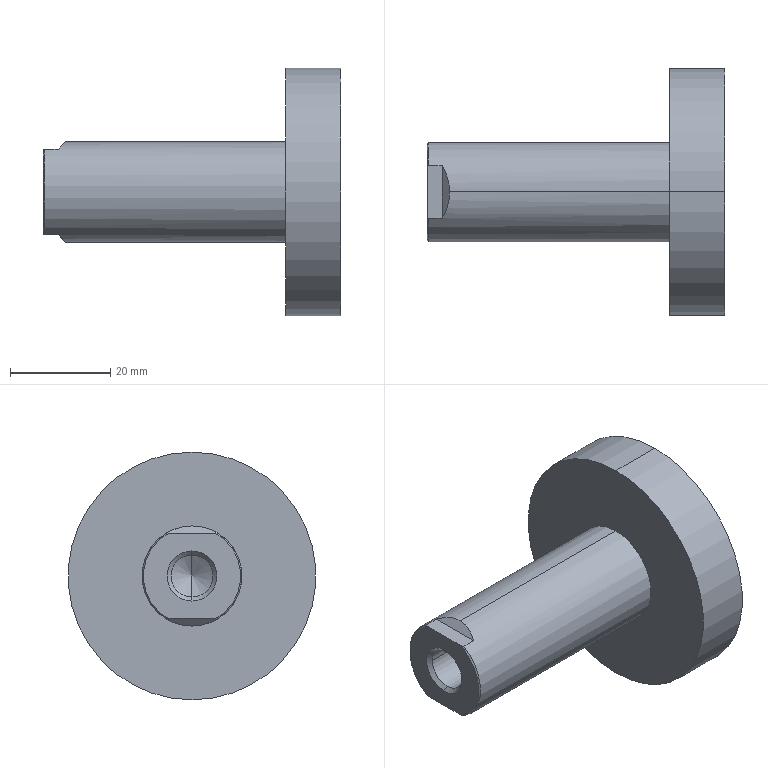Part | SolidWorks | features BaseBody 1 | 1 solid | 19 faces | box 59.5 x 49.5 x 49.5 mm | volume 35281 mm3 | plane 7 | cylinder 6 | cone 6 | commonest cylinder face diameters 8.376 x2 20 x2 49.5 x2
STEP:
#1=CARTESIAN_POINT('',(39.5,0.,10.));
#2=VERTEX_POINT('',#1);
#3=CARTESIAN_POINT('',(39.5,0.,-10.));
#4=VERTEX_POINT('',#3);
#5=CARTESIAN_POINT('',(39.5,0.,0.));
#6=DIRECTION('',(-1.,0.,0.));
#7=DIRECTION('',(0.,0.,1.));
#8=AXIS2_PLACEMENT_3D('',#5,#6,#7);
#9=CIRCLE('',#8,10.);
#10=EDGE_CURVE('',#2,#4,#9,.T.);
#11=ORIENTED_EDGE('',*,*,#10,.T.);
#12=CARTESIAN_POINT('',(-4.5,0.,-10.));
#13=VERTEX_POINT('',#12);
#14=CARTESIAN_POINT('',(0.,0.,-10.));
#15=DIRECTION('',(-1.,0.,0.));
#16=VECTOR('',#15,1000.);
#17=LINE('',#14,#16);
#18=EDGE_CURVE('',#4,#13,#17,.T.);
#19=ORIENTED_EDGE('',*,*,#18,.T.);
#20=CARTESIAN_POINT('',(-6.,5.268,-8.5));
#21=VERTEX_POINT('',#20);
#22=CARTESIAN_POINT('',(-4.5,0.,-10.));
#23=CARTESIAN_POINT('',(-4.5,1.873,-10.));
#24=CARTESIAN_POINT('',(-5.013,3.675,-9.487));
#25=CARTESIAN_POINT('',(-6.,5.268,-8.5));
#26=(BOUNDED_CURVE()B_SPLINE_CURVE(3,(#22,#23,#24,#25),.UNSPECIFIED.,.F.,.F.)B_SPLINE_CURVE_WITH_KNOTS((4,4),(3.142,3.696),.UNSPECIFIED.)CURVE()GEOMETRIC_REPRESENTATION_ITEM()RATIONAL_B_SPLINE_CURVE((1.,0.9745,0.9745,1.))REPRESENTATION_ITEM(''));
#27=EDGE_CURVE('',#13,#21,#26,.T.);
#28=ORIENTED_EDGE('',*,*,#27,.T.);
#29=CARTESIAN_POINT('',(-8.75,5.268,-8.5));
#30=VERTEX_POINT('',#29);
#31=CARTESIAN_POINT('',(0.,5.268,-8.5));
#32=DIRECTION('',(-1.,0.,0.));
#33=VECTOR('',#32,1000.);
#34=LINE('',#31,#33);
#35=EDGE_CURVE('',#21,#30,#34,.T.);
#36=ORIENTED_EDGE('',*,*,#35,.T.);
#37=CARTESIAN_POINT('',(-8.75,5.268,8.5));
#38=VERTEX_POINT('',#37);
#39=CARTESIAN_POINT('',(-8.75,0.,0.));
#40=DIRECTION('',(1.,0.,0.));
#41=DIRECTION('',(0.,0.,1.));
#42=AXIS2_PLACEMENT_3D('',#39,#40,#41);
#43=CIRCLE('',#42,10.);
#44=EDGE_CURVE('',#30,#38,#43,.T.);
#45=ORIENTED_EDGE('',*,*,#44,.T.);
#46=CARTESIAN_POINT('',(-6.,5.268,8.5));
#47=VERTEX_POINT('',#46);
#48=CARTESIAN_POINT('',(0.,5.268,8.5));
#49=DIRECTION('',(1.,0.,0.));
#50=VECTOR('',#49,1000.);
#51=LINE('',#48,#50);
#52=EDGE_CURVE('',#38,#47,#51,.T.);
#53=ORIENTED_EDGE('',*,*,#52,.T.);
#54=CARTESIAN_POINT('',(-4.5,0.,10.));
#55=VERTEX_POINT('',#54);
#56=CARTESIAN_POINT('',(-6.,5.268,8.5));
#57=CARTESIAN_POINT('',(-5.013,3.675,9.487));
#58=CARTESIAN_POINT('',(-4.5,1.873,10.));
#59=CARTESIAN_POINT('',(-4.5,0.,10.));
#60=(BOUNDED_CURVE()B_SPLINE_CURVE(3,(#56,#57,#58,#59),.UNSPECIFIED.,.F.,.F.)B_SPLINE_CURVE_WITH_KNOTS((4,4),(2.587,3.142),.UNSPECIFIED.)CURVE()GEOMETRIC_REPRESENTATION_ITEM()RATIONAL_B_SPLINE_CURVE((1.,0.9745,0.9745,1.))REPRESENTATION_ITEM(''));
#61=EDGE_CURVE('',#47,#55,#60,.T.);
#62=ORIENTED_EDGE('',*,*,#61,.T.);
#63=CARTESIAN_POINT('',(0.,0.,10.));
#64=DIRECTION('',(-1.,0.,0.));
#65=VECTOR('',#64,1000.);
#66=LINE('',#63,#65);
#67=EDGE_CURVE('',#2,#55,#66,.T.);
#68=ORIENTED_EDGE('',*,*,#67,.F.);
#69=EDGE_LOOP('',(#11,#19,#28,#36,#45,#53,#62,#68));
#70=FACE_OUTER_BOUND('',#69,.T.);
#71=CARTESIAN_POINT('',(0.,0.,0.));
#72=DIRECTION('',(-1.,0.,0.));
#73=DIRECTION('',(0.,0.,1.));
#74=AXIS2_PLACEMENT_3D('',#71,#72,#73);
#75=CYLINDRICAL_SURFACE('',#74,10.);
#76=ADVANCED_FACE('',(#70),#75,.T.);
#77=CARTESIAN_POINT('',(50.5,0.,24.75));
#78=VERTEX_POINT('',#77);
#79=CARTESIAN_POINT('',(50.5,0.,-24.75));
#80=VERTEX_POINT('',#79);
#81=CARTESIAN_POINT('',(50.5,0.,0.));
#82=DIRECTION('',(-1.,0.,0.));
#83=DIRECTION('',(0.,0.,1.));
#84=AXIS2_PLACEMENT_3D('',#81,#82,#83);
#85=CIRCLE('',#84,24.75);
#86=EDGE_CURVE('',#78,#80,#85,.T.);
#87=ORIENTED_EDGE('',*,*,#86,.T.);
#88=CARTESIAN_POINT('',(39.5,0.,-24.75));
#89=VERTEX_POINT('',#88);
#90=CARTESIAN_POINT('',(50.5,0.,-24.75));
#91=DIRECTION('',(-1.,0.,0.));
#92=VECTOR('',#91,1000.);
#93=LINE('',#90,#92);
#94=EDGE_CURVE('',#80,#89,#93,.T.);
#95=ORIENTED_EDGE('',*,*,#94,.T.);
#96=CARTESIAN_POINT('',(39.5,0.,24.75));
#97=VERTEX_POINT('',#96);
#98=CARTESIAN_POINT('',(39.5,0.,0.));
#99=DIRECTION('',(1.,0.,0.));
#100=DIRECTION('',(0.,0.,1.));
#101=AXIS2_PLACEMENT_3D('',#98,#99,#100);
#102=CIRCLE('',#101,24.75);
#103=EDGE_CURVE('',#89,#97,#102,.T.);
#104=ORIENTED_EDGE('',*,*,#103,.T.);
#105=CARTESIAN_POINT('',(50.5,0.,24.75));
#106=DIRECTION('',(-1.,0.,0.));
#107=VECTOR('',#106,1000.);
#108=LINE('',#105,#107);
#109=EDGE_CURVE('',#78,#97,#108,.T.);
#110=ORIENTED_EDGE('',*,*,#109,.F.);
#111=EDGE_LOOP('',(#87,#95,#104,#110));
#112=FACE_OUTER_BOUND('',#111,.T.);
#113=CARTESIAN_POINT('',(50.5,0.,0.));
#114=DIRECTION('',(-1.,0.,0.));
#115=DIRECTION('',(0.,0.,1.));
#116=AXIS2_PLACEMENT_3D('',#113,#114,#115);
#117=CYLINDRICAL_SURFACE('',#116,24.75);
#118=ADVANCED_FACE('',(#112),#117,.T.);
#119=CARTESIAN_POINT('',(-8.188,0.,-4.188));
#120=VERTEX_POINT('',#119);
#121=CARTESIAN_POINT('',(-8.188,-4.188,0.));
#122=VERTEX_POINT('',#121);
#123=CARTESIAN_POINT('',(-8.188,0.,0.));
#124=DIRECTION('',(-1.,0.,0.));
#125=DIRECTION('',(0.,-1.,0.));
#126=AXIS2_PLACEMENT_3D('',#123,#124,#125);
#127=CIRCLE('',#126,4.188);
#128=EDGE_CURVE('',#120,#122,#127,.T.);
#129=ORIENTED_EDGE('',*,*,#128,.F.);
#130=CARTESIAN_POINT('',(-9.,0.,-5.));
#131=VERTEX_POINT('',#130);
#132=CARTESIAN_POINT('',(-9.,0.,-5.));
#133=DIRECTION('',(-0.7071,0.,-0.7071));
#134=VECTOR('',#133,1000.);
#135=LINE('',#132,#134);
#136=EDGE_CURVE('',#120,#131,#135,.T.);
#137=ORIENTED_EDGE('',*,*,#136,.T.);
#138=CARTESIAN_POINT('',(-9.,0.,5.));
#139=VERTEX_POINT('',#138);
#140=CARTESIAN_POINT('',(-9.,0.,0.));
#141=DIRECTION('',(-1.,0.,0.));
#142=DIRECTION('',(0.,0.,1.));
#143=AXIS2_PLACEMENT_3D('',#140,#141,#142);
#144=CIRCLE('',#143,5.);
#145=EDGE_CURVE('',#131,#139,#144,.T.);
#146=ORIENTED_EDGE('',*,*,#145,.T.);
#147=CARTESIAN_POINT('',(-8.188,0.,4.188));
#148=VERTEX_POINT('',#147);
#149=CARTESIAN_POINT('',(-9.,0.,5.));
#150=DIRECTION('',(-0.7071,0.,0.7071));
#151=VECTOR('',#150,1000.);
#152=LINE('',#149,#151);
#153=EDGE_CURVE('',#148,#139,#152,.T.);
#154=ORIENTED_EDGE('',*,*,#153,.F.);
#155=CARTESIAN_POINT('',(-8.188,0.,0.));
#156=DIRECTION('',(-1.,0.,0.));
#157=DIRECTION('',(0.,-1.,0.));
#158=AXIS2_PLACEMENT_3D('',#155,#156,#157);
#159=CIRCLE('',#158,4.188);
#160=EDGE_CURVE('',#122,#148,#159,.T.);
#161=ORIENTED_EDGE('',*,*,#160,.F.);
#162=EDGE_LOOP('',(#129,#137,#146,#154,#161));
#163=FACE_OUTER_BOUND('',#162,.T.);
#164=CARTESIAN_POINT('',(-9.,0.,0.));
#165=DIRECTION('',(-1.,0.,0.));
#166=DIRECTION('',(0.,0.,1.));
#167=AXIS2_PLACEMENT_3D('',#164,#165,#166);
#168=CONICAL_SURFACE('',#167,5.,0.7854);
#169=ADVANCED_FACE('',(#163),#168,.F.);
#170=CARTESIAN_POINT('',(9.,4.188,0.));
#171=VERTEX_POINT('',#170);
#172=CARTESIAN_POINT('',(9.,0.,-4.188));
#173=VERTEX_POINT('',#172);
#174=CARTESIAN_POINT('',(9.,0.,0.));
#175=DIRECTION('',(-1.,0.,0.));
#176=DIRECTION('',(0.,-1.,0.));
#177=AXIS2_PLACEMENT_3D('',#174,#175,#176);
#178=CIRCLE('',#177,4.188);
#179=EDGE_CURVE('',#171,#173,#178,.T.);
#180=ORIENTED_EDGE('',*,*,#179,.F.);
#181=CARTESIAN_POINT('',(-8.188,4.188,0.));
#182=VERTEX_POINT('',#181);
#183=CARTESIAN_POINT('',(11.418,4.188,0.));
#184=DIRECTION('',(-1.,0.,0.));
#185=VECTOR('',#184,1000.);
#186=LINE('',#183,#185);
#187=EDGE_CURVE('',#171,#182,#186,.T.);
#188=ORIENTED_EDGE('',*,*,#187,.T.);
#189=CARTESIAN_POINT('',(-8.188,0.,0.));
#190=DIRECTION('',(-1.,0.,0.));
#191=DIRECTION('',(0.,-1.,0.));
#192=AXIS2_PLACEMENT_3D('',#189,#190,#191);
#193=CIRCLE('',#192,4.188);
#194=EDGE_CURVE('',#182,#120,#193,.T.);
#195=ORIENTED_EDGE('',*,*,#194,.T.);
#196=ORIENTED_EDGE('',*,*,#128,.T.);
#197=CARTESIAN_POINT('',(9.,-4.188,0.));
#198=VERTEX_POINT('',#197);
#199=CARTESIAN_POINT('',(11.418,-4.188,0.));
#200=DIRECTION('',(-1.,0.,0.));
#201=VECTOR('',#200,1000.);
#202=LINE('',#199,#201);
#203=EDGE_CURVE('',#198,#122,#202,.T.);
#204=ORIENTED_EDGE('',*,*,#203,.F.);
#205=CARTESIAN_POINT('',(9.,0.,0.));
#206=DIRECTION('',(-1.,0.,0.));
#207=DIRECTION('',(0.,-1.,0.));
#208=AXIS2_PLACEMENT_3D('',#205,#206,#207);
#209=CIRCLE('',#208,4.188);
#210=EDGE_CURVE('',#173,#198,#209,.T.);
#211=ORIENTED_EDGE('',*,*,#210,.F.);
#212=EDGE_LOOP('',(#180,#188,#195,#196,#204,#211));
#213=FACE_OUTER_BOUND('',#212,.T.);
#214=CARTESIAN_POINT('',(11.418,0.,0.));
#215=DIRECTION('',(-1.,0.,0.));
#216=DIRECTION('',(0.,-1.,0.));
#217=AXIS2_PLACEMENT_3D('',#214,#215,#216);
#218=CYLINDRICAL_SURFACE('',#217,4.188);
#219=ADVANCED_FACE('',(#213),#218,.F.);
#220=CARTESIAN_POINT('',(11.418,0.,0.));
#221=VERTEX_POINT('',#220);
#222=CARTESIAN_POINT('',(9.,0.,4.188));
#223=VERTEX_POINT('',#222);
#224=CARTESIAN_POINT('',(9.,0.,4.188));
#225=DIRECTION('',(-0.5,0.,0.866));
#226=VECTOR('',#225,1000.);
#227=LINE('',#224,#226);
#228=EDGE_CURVE('',#221,#223,#227,.T.);
#229=ORIENTED_EDGE('',*,*,#228,.F.);
#230=CARTESIAN_POINT('',(9.,0.,-4.188));
#231=DIRECTION('',(-0.5,0.,-0.866));
#232=VECTOR('',#231,1000.);
#233=LINE('',#230,#232);
#234=EDGE_CURVE('',#221,#173,#233,.T.);
#235=ORIENTED_EDGE('',*,*,#234,.T.);
#236=ORIENTED_EDGE('',*,*,#210,.T.);
#237=CARTESIAN_POINT('',(9.,0.,0.));
#238=DIRECTION('',(-1.,0.,0.));
#239=DIRECTION('',(0.,-1.,0.));
#240=AXIS2_PLACEMENT_3D('',#237,#238,#239);
#241=CIRCLE('',#240,4.188);
#242=EDGE_CURVE('',#198,#223,#241,.T.);
#243=ORIENTED_EDGE('',*,*,#242,.T.);
#244=EDGE_LOOP('',(#229,#235,#236,#243));
#245=FACE_OUTER_BOUND('',#244,.T.);
#246=CARTESIAN_POINT('',(9.,0.,0.));
#247=DIRECTION('',(-1.,0.,0.));
#248=DIRECTION('',(0.,0.,1.));
#249=AXIS2_PLACEMENT_3D('',#246,#247,#248);
#250=CONICAL_SURFACE('',#249,4.188,1.047);
#251=ADVANCED_FACE('',(#245),#250,.F.);
#252=ORIENTED_EDGE('',*,*,#18,.F.);
#253=CARTESIAN_POINT('',(39.5,0.,0.));
#254=DIRECTION('',(-1.,0.,0.));
#255=DIRECTION('',(0.,0.,1.));
#256=AXIS2_PLACEMENT_3D('',#253,#254,#255);
#257=CIRCLE('',#256,10.);
#258=EDGE_CURVE('',#4,#2,#257,.T.);
#259=ORIENTED_EDGE('',*,*,#258,.T.);
#260=ORIENTED_EDGE('',*,*,#67,.T.);
#261=CARTESIAN_POINT('',(-6.,-5.268,8.5));
#262=VERTEX_POINT('',#261);
#263=CARTESIAN_POINT('',(-4.5,0.,10.));
#264=CARTESIAN_POINT('',(-4.5,-1.873,10.));
#265=CARTESIAN_POINT('',(-5.013,-3.675,9.487));
#266=CARTESIAN_POINT('',(-6.,-5.268,8.5));
#267=(BOUNDED_CURVE()B_SPLINE_CURVE(3,(#263,#264,#265,#266),.UNSPECIFIED.,.F.,.F.)B_SPLINE_CURVE_WITH_KNOTS((4,4),(3.142,3.696),.UNSPECIFIED.)CURVE()GEOMETRIC_REPRESENTATION_ITEM()RATIONAL_B_SPLINE_CURVE((1.,0.9745,0.9745,1.))REPRESENTATION_ITEM(''));
#268=EDGE_CURVE('',#55,#262,#267,.T.);
#269=ORIENTED_EDGE('',*,*,#268,.T.);
#270=CARTESIAN_POINT('',(-8.75,-5.268,8.5));
#271=VERTEX_POINT('',#270);
#272=CARTESIAN_POINT('',(0.,-5.268,8.5));
#273=DIRECTION('',(-1.,0.,0.));
#274=VECTOR('',#273,1000.);
#275=LINE('',#272,#274);
#276=EDGE_CURVE('',#262,#271,#275,.T.);
#277=ORIENTED_EDGE('',*,*,#276,.T.);
#278=CARTESIAN_POINT('',(-8.75,-5.268,-8.5));
#279=VERTEX_POINT('',#278);
#280=CARTESIAN_POINT('',(-8.75,0.,0.));
#281=DIRECTION('',(1.,0.,0.));
#282=DIRECTION('',(0.,0.,1.));
#283=AXIS2_PLACEMENT_3D('',#280,#281,#282);
#284=CIRCLE('',#283,10.);
#285=EDGE_CURVE('',#271,#279,#284,.T.);
#286=ORIENTED_EDGE('',*,*,#285,.T.);
#287=CARTESIAN_POINT('',(-6.,-5.268,-8.5));
#288=VERTEX_POINT('',#287);
#289=CARTESIAN_POINT('',(0.,-5.268,-8.5));
#290=DIRECTION('',(1.,0.,0.));
#291=VECTOR('',#290,1000.);
#292=LINE('',#289,#291);
#293=EDGE_CURVE('',#279,#288,#292,.T.);
#294=ORIENTED_EDGE('',*,*,#293,.T.);
#295=CARTESIAN_POINT('',(-6.,-5.268,-8.5));
#296=CARTESIAN_POINT('',(-5.013,-3.675,-9.487));
#297=CARTESIAN_POINT('',(-4.5,-1.873,-10.));
#298=CARTESIAN_POINT('',(-4.5,0.,-10.));
#299=(BOUNDED_CURVE()B_SPLINE_CURVE(3,(#295,#296,#297,#298),.UNSPECIFIED.,.F.,.F.)B_SPLINE_CURVE_WITH_KNOTS((4,4),(2.587,3.142),.UNSPECIFIED.)CURVE()GEOMETRIC_REPRESENTATION_ITEM()RATIONAL_B_SPLINE_CURVE((1.,0.9745,0.9745,1.))REPRESENTATION_ITEM(''));
#300=EDGE_CURVE('',#288,#13,#299,.T.);
#301=ORIENTED_EDGE('',*,*,#300,.T.);
#302=EDGE_LOOP('',(#252,#259,#260,#269,#277,#286,#294,#301));
#303=FACE_OUTER_BOUND('',#302,.T.);
#304=CARTESIAN_POINT('',(0.,0.,0.));
#305=DIRECTION('',(-1.,0.,0.));
#306=DIRECTION('',(0.,0.,1.));
#307=AXIS2_PLACEMENT_3D('',#304,#305,#306);
#308=CYLINDRICAL_SURFACE('',#307,10.);
#309=ADVANCED_FACE('',(#303),#308,.T.);
#310=ORIENTED_EDGE('',*,*,#61,.F.);
#311=CARTESIAN_POINT('',(-6.,17.,8.5));
#312=DIRECTION('',(0.,-1.,0.));
#313=VECTOR('',#312,1000.);
#314=LINE('',#311,#313);
#315=EDGE_CURVE('',#47,#262,#314,.T.);
#316=ORIENTED_EDGE('',*,*,#315,.T.);
#317=ORIENTED_EDGE('',*,*,#268,.F.);
#318=EDGE_LOOP('',(#310,#316,#317));
#319=FACE_OUTER_BOUND('',#318,.T.);
#320=CARTESIAN_POINT('',(-1.,17.,13.5));
#321=DIRECTION('',(-0.7071,0.,0.7071));
#322=DIRECTION('',(0.7071,0.,0.7071));
#323=AXIS2_PLACEMENT_3D('',#320,#321,#322);
#324=PLANE('',#323);
#325=ADVANCED_FACE('',(#319),#324,.T.);
#326=CARTESIAN_POINT('',(-9.,4.776,8.5));
#327=VERTEX_POINT('',#326);
#328=CARTESIAN_POINT('',(-8.75,5.268,8.5));
#329=CARTESIAN_POINT('',(-8.837,5.102,8.5));
#330=CARTESIAN_POINT('',(-8.921,4.938,8.5));
#331=CARTESIAN_POINT('',(-9.,4.776,8.5));
#332=B_SPLINE_CURVE_WITH_KNOTS('',3,(#328,#329,#330,#331),.UNSPECIFIED.,.F.,.F.,(4,4),(0.,1.),.UNSPECIFIED.);
#333=EDGE_CURVE('',#38,#327,#332,.T.);
#334=ORIENTED_EDGE('',*,*,#333,.T.);
#335=CARTESIAN_POINT('',(-9.,-4.776,8.5));
#336=VERTEX_POINT('',#335);
#337=CARTESIAN_POINT('',(-9.,17.,8.5));
#338=DIRECTION('',(0.,-1.,0.));
#339=VECTOR('',#338,1000.);
#340=LINE('',#337,#339);
#341=EDGE_CURVE('',#327,#336,#340,.T.);
#342=ORIENTED_EDGE('',*,*,#341,.T.);
#343=CARTESIAN_POINT('',(-9.,-4.776,8.5));
#344=CARTESIAN_POINT('',(-8.921,-4.938,8.5));
#345=CARTESIAN_POINT('',(-8.837,-5.102,8.5));
#346=CARTESIAN_POINT('',(-8.75,-5.268,8.5));
#347=B_SPLINE_CURVE_WITH_KNOTS('',3,(#343,#344,#345,#346),.UNSPECIFIED.,.F.,.F.,(4,4),(0.,1.),.UNSPECIFIED.);
#348=EDGE_CURVE('',#336,#271,#347,.T.);
#349=ORIENTED_EDGE('',*,*,#348,.T.);
#350=ORIENTED_EDGE('',*,*,#276,.F.);
#351=ORIENTED_EDGE('',*,*,#315,.F.);
#352=ORIENTED_EDGE('',*,*,#52,.F.);
#353=EDGE_LOOP('',(#334,#342,#349,#350,#351,#352));
#354=FACE_OUTER_BOUND('',#353,.T.);
#355=CARTESIAN_POINT('',(-6.,17.,8.5));
#356=DIRECTION('',(0.,0.,1.));
#357=DIRECTION('',(1.,0.,0.));
#358=AXIS2_PLACEMENT_3D('',#355,#356,#357);
#359=PLANE('',#358);
#360=ADVANCED_FACE('',(#354),#359,.T.);
#361=ORIENTED_EDGE('',*,*,#333,.F.);
#362=ORIENTED_EDGE('',*,*,#44,.F.);
#363=CARTESIAN_POINT('',(-9.,4.776,-8.5));
#364=VERTEX_POINT('',#363);
#365=CARTESIAN_POINT('',(-8.75,5.268,-8.5));
#366=CARTESIAN_POINT('',(-8.837,5.103,-8.5));
#367=CARTESIAN_POINT('',(-8.92,4.939,-8.5));
#368=CARTESIAN_POINT('',(-9.,4.776,-8.5));
#369=B_SPLINE_CURVE_WITH_KNOTS('',3,(#365,#366,#367,#368),.UNSPECIFIED.,.F.,.F.,(4,4),(0.,1.),.UNSPECIFIED.);
#370=EDGE_CURVE('',#30,#364,#369,.T.);
#371=ORIENTED_EDGE('',*,*,#370,.T.);
#372=CARTESIAN_POINT('',(-9.,0.,0.));
#373=DIRECTION('',(1.,0.,0.));
#374=DIRECTION('',(0.,0.,-1.));
#375=AXIS2_PLACEMENT_3D('',#372,#373,#374);
#376=CIRCLE('',#375,9.75);
#377=EDGE_CURVE('',#364,#327,#376,.T.);
#378=ORIENTED_EDGE('',*,*,#377,.T.);
#379=EDGE_LOOP('',(#361,#362,#371,#378));
#380=FACE_OUTER_BOUND('',#379,.T.);
#381=CARTESIAN_POINT('',(-8.75,0.,0.));
#382=DIRECTION('',(1.,0.,0.));
#383=DIRECTION('',(0.,0.,-1.));
#384=AXIS2_PLACEMENT_3D('',#381,#382,#383);
#385=CONICAL_SURFACE('',#384,10.,0.7854);
#386=ADVANCED_FACE('',(#380),#385,.T.);
#387=CARTESIAN_POINT('',(-9.,-4.776,-8.5));
#388=VERTEX_POINT('',#387);
#389=CARTESIAN_POINT('',(-8.75,-5.268,-8.5));
#390=CARTESIAN_POINT('',(-8.837,-5.102,-8.5));
#391=CARTESIAN_POINT('',(-8.921,-4.938,-8.5));
#392=CARTESIAN_POINT('',(-9.,-4.776,-8.5));
#393=B_SPLINE_CURVE_WITH_KNOTS('',3,(#389,#390,#391,#392),.UNSPECIFIED.,.F.,.F.,(4,4),(0.,1.),.UNSPECIFIED.);
#394=EDGE_CURVE('',#279,#388,#393,.T.);
#395=ORIENTED_EDGE('',*,*,#394,.T.);
#396=CARTESIAN_POINT('',(-9.,17.,-8.5));
#397=DIRECTION('',(0.,1.,0.));
#398=VECTOR('',#397,1000.);
#399=LINE('',#396,#398);
#400=EDGE_CURVE('',#388,#364,#399,.T.);
#401=ORIENTED_EDGE('',*,*,#400,.T.);
#402=ORIENTED_EDGE('',*,*,#370,.F.);
#403=ORIENTED_EDGE('',*,*,#35,.F.);
#404=CARTESIAN_POINT('',(-6.,17.,-8.5));
#405=DIRECTION('',(0.,-1.,0.));
#406=VECTOR('',#405,1000.);
#407=LINE('',#404,#406);
#408=EDGE_CURVE('',#21,#288,#407,.T.);
#409=ORIENTED_EDGE('',*,*,#408,.T.);
#410=ORIENTED_EDGE('',*,*,#293,.F.);
#411=EDGE_LOOP('',(#395,#401,#402,#403,#409,#410));
#412=FACE_OUTER_BOUND('',#411,.T.);
#413=CARTESIAN_POINT('',(-9.,17.,-8.5));
#414=DIRECTION('',(0.,0.,-1.));
#415=DIRECTION('',(-1.,0.,0.));
#416=AXIS2_PLACEMENT_3D('',#413,#414,#415);
#417=PLANE('',#416);
#418=ADVANCED_FACE('',(#412),#417,.T.);
#419=ORIENTED_EDGE('',*,*,#300,.F.);
#420=ORIENTED_EDGE('',*,*,#408,.F.);
#421=ORIENTED_EDGE('',*,*,#27,.F.);
#422=EDGE_LOOP('',(#419,#420,#421));
#423=FACE_OUTER_BOUND('',#422,.T.);
#424=CARTESIAN_POINT('',(-6.,17.,-8.5));
#425=DIRECTION('',(-0.7071,0.,-0.7071));
#426=DIRECTION('',(-0.7071,0.,0.7071));
#427=AXIS2_PLACEMENT_3D('',#424,#425,#426);
#428=PLANE('',#427);
#429=ADVANCED_FACE('',(#423),#428,.T.);
#430=ORIENTED_EDGE('',*,*,#394,.F.);
#431=ORIENTED_EDGE('',*,*,#285,.F.);
#432=ORIENTED_EDGE('',*,*,#348,.F.);
#433=CARTESIAN_POINT('',(-9.,0.,0.));
#434=DIRECTION('',(1.,0.,0.));
#435=DIRECTION('',(0.,0.,-1.));
#436=AXIS2_PLACEMENT_3D('',#433,#434,#435);
#437=CIRCLE('',#436,9.75);
#438=EDGE_CURVE('',#336,#388,#437,.T.);
#439=ORIENTED_EDGE('',*,*,#438,.T.);
#440=EDGE_LOOP('',(#430,#431,#432,#439));
#441=FACE_OUTER_BOUND('',#440,.T.);
#442=CARTESIAN_POINT('',(-8.75,0.,0.));
#443=DIRECTION('',(1.,0.,0.));
#444=DIRECTION('',(0.,0.,-1.));
#445=AXIS2_PLACEMENT_3D('',#442,#443,#444);
#446=CONICAL_SURFACE('',#445,10.,0.7854);
#447=ADVANCED_FACE('',(#441),#446,.T.);
#448=ORIENTED_EDGE('',*,*,#10,.F.);
#449=ORIENTED_EDGE('',*,*,#258,.F.);
#450=EDGE_LOOP('',(#448,#449));
#451=FACE_BOUND('',#450,.T.);
#452=CARTESIAN_POINT('',(39.5,0.,0.));
#453=DIRECTION('',(1.,0.,0.));
#454=DIRECTION('',(0.,0.,1.));
#455=AXIS2_PLACEMENT_3D('',#452,#453,#454);
#456=CIRCLE('',#455,24.75);
#457=EDGE_CURVE('',#97,#89,#456,.T.);
#458=ORIENTED_EDGE('',*,*,#457,.F.);
#459=ORIENTED_EDGE('',*,*,#103,.F.);
#460=EDGE_LOOP('',(#458,#459));
#461=FACE_OUTER_BOUND('',#460,.T.);
#462=CARTESIAN_POINT('',(39.5,10.,0.));
#463=DIRECTION('',(1.,0.,0.));
#464=DIRECTION('',(0.,0.,-1.));
#465=AXIS2_PLACEMENT_3D('',#462,#463,#464);
#466=PLANE('',#465);
#467=ADVANCED_FACE('',(#451,#461),#466,.F.);
#468=CARTESIAN_POINT('',(-9.,0.,0.));
#469=DIRECTION('',(-1.,0.,0.));
#470=DIRECTION('',(0.,0.,1.));
#471=AXIS2_PLACEMENT_3D('',#468,#469,#470);
#472=CIRCLE('',#471,5.);
#473=EDGE_CURVE('',#139,#131,#472,.T.);
#474=ORIENTED_EDGE('',*,*,#473,.F.);
#475=ORIENTED_EDGE('',*,*,#145,.F.);
#476=EDGE_LOOP('',(#474,#475));
#477=FACE_BOUND('',#476,.T.);
#478=ORIENTED_EDGE('',*,*,#400,.F.);
#479=ORIENTED_EDGE('',*,*,#438,.F.);
#480=ORIENTED_EDGE('',*,*,#341,.F.);
#481=ORIENTED_EDGE('',*,*,#377,.F.);
#482=EDGE_LOOP('',(#478,#479,#480,#481));
#483=FACE_OUTER_BOUND('',#482,.T.);
#484=CARTESIAN_POINT('',(-9.,0.,0.));
#485=DIRECTION('',(1.,0.,0.));
#486=DIRECTION('',(0.,0.,-1.));
#487=AXIS2_PLACEMENT_3D('',#484,#485,#486);
#488=PLANE('',#487);
#489=ADVANCED_FACE('',(#477,#483),#488,.F.);
#490=ORIENTED_EDGE('',*,*,#94,.F.);
#491=CARTESIAN_POINT('',(50.5,0.,0.));
#492=DIRECTION('',(-1.,0.,0.));
#493=DIRECTION('',(0.,0.,1.));
#494=AXIS2_PLACEMENT_3D('',#491,#492,#493);
#495=CIRCLE('',#494,24.75);
#496=EDGE_CURVE('',#80,#78,#495,.T.);
#497=ORIENTED_EDGE('',*,*,#496,.T.);
#498=ORIENTED_EDGE('',*,*,#109,.T.);
#499=ORIENTED_EDGE('',*,*,#457,.T.);
#500=EDGE_LOOP('',(#490,#497,#498,#499));
#501=FACE_OUTER_BOUND('',#500,.T.);
#502=CARTESIAN_POINT('',(50.5,0.,0.));
#503=DIRECTION('',(-1.,0.,0.));
#504=DIRECTION('',(0.,0.,1.));
#505=AXIS2_PLACEMENT_3D('',#502,#503,#504);
#506=CYLINDRICAL_SURFACE('',#505,24.75);
#507=ADVANCED_FACE('',(#501),#506,.T.);
#508=ORIENTED_EDGE('',*,*,#136,.F.);
#509=ORIENTED_EDGE('',*,*,#194,.F.);
#510=CARTESIAN_POINT('',(-8.188,0.,0.));
#511=DIRECTION('',(-1.,0.,0.));
#512=DIRECTION('',(0.,-1.,0.));
#513=AXIS2_PLACEMENT_3D('',#510,#511,#512);
#514=CIRCLE('',#513,4.188);
#515=EDGE_CURVE('',#148,#182,#514,.T.);
#516=ORIENTED_EDGE('',*,*,#515,.F.);
#517=ORIENTED_EDGE('',*,*,#153,.T.);
#518=ORIENTED_EDGE('',*,*,#473,.T.);
#519=EDGE_LOOP('',(#508,#509,#516,#517,#518));
#520=FACE_OUTER_BOUND('',#519,.T.);
#521=CARTESIAN_POINT('',(-9.,0.,0.));
#522=DIRECTION('',(-1.,0.,0.));
#523=DIRECTION('',(0.,0.,1.));
#524=AXIS2_PLACEMENT_3D('',#521,#522,#523);
#525=CONICAL_SURFACE('',#524,5.,0.7854);
#526=ADVANCED_FACE('',(#520),#525,.F.);
#527=ORIENTED_EDGE('',*,*,#86,.F.);
#528=ORIENTED_EDGE('',*,*,#496,.F.);
#529=EDGE_LOOP('',(#527,#528));
#530=FACE_OUTER_BOUND('',#529,.T.);
#531=CARTESIAN_POINT('',(50.5,24.75,0.));
#532=DIRECTION('',(-1.,0.,0.));
#533=DIRECTION('',(0.,0.,1.));
#534=AXIS2_PLACEMENT_3D('',#531,#532,#533);
#535=PLANE('',#534);
#536=ADVANCED_FACE('',(#530),#535,.F.);
#537=ORIENTED_EDGE('',*,*,#187,.F.);
#538=CARTESIAN_POINT('',(9.,0.,0.));
#539=DIRECTION('',(-1.,0.,0.));
#540=DIRECTION('',(0.,-1.,0.));
#541=AXIS2_PLACEMENT_3D('',#538,#539,#540);
#542=CIRCLE('',#541,4.188);
#543=EDGE_CURVE('',#223,#171,#542,.T.);
#544=ORIENTED_EDGE('',*,*,#543,.F.);
#545=ORIENTED_EDGE('',*,*,#242,.F.);
#546=ORIENTED_EDGE('',*,*,#203,.T.);
#547=ORIENTED_EDGE('',*,*,#160,.T.);
#548=ORIENTED_EDGE('',*,*,#515,.T.);
#549=EDGE_LOOP('',(#537,#544,#545,#546,#547,#548));
#550=FACE_OUTER_BOUND('',#549,.T.);
#551=CARTESIAN_POINT('',(11.418,0.,0.));
#552=DIRECTION('',(-1.,0.,0.));
#553=DIRECTION('',(0.,-1.,0.));
#554=AXIS2_PLACEMENT_3D('',#551,#552,#553);
#555=CYLINDRICAL_SURFACE('',#554,4.188);
#556=ADVANCED_FACE('',(#550),#555,.F.);
#557=ORIENTED_EDGE('',*,*,#234,.F.);
#558=ORIENTED_EDGE('',*,*,#228,.T.);
#559=ORIENTED_EDGE('',*,*,#543,.T.);
#560=ORIENTED_EDGE('',*,*,#179,.T.);
#561=EDGE_LOOP('',(#557,#558,#559,#560));
#562=FACE_OUTER_BOUND('',#561,.T.);
#563=CARTESIAN_POINT('',(9.,0.,0.));
#564=DIRECTION('',(-1.,0.,0.));
#565=DIRECTION('',(0.,0.,1.));
#566=AXIS2_PLACEMENT_3D('',#563,#564,#565);
#567=CONICAL_SURFACE('',#566,4.188,1.047);
#568=ADVANCED_FACE('',(#562),#567,.F.);
#569=CLOSED_SHELL('',(#76,#118,#169,#219,#251,#309,#325,#360,#386,#418,#429,#447,#467,#489,#507,#526,#536,#556,#568));
#570=MANIFOLD_SOLID_BREP('',#569);
#571=CARTESIAN_POINT('',(0.,0.,0.));
#572=DIRECTION('',(0.,0.,1.));
#573=DIRECTION('',(1.,0.,0.));
#574=AXIS2_PLACEMENT_3D('',#571,#572,#573);
#575=(LENGTH_UNIT()NAMED_UNIT(*)SI_UNIT(.MILLI.,.METRE.));
#576=UNCERTAINTY_MEASURE_WITH_UNIT(LENGTH_MEASURE(0.00001),#575,'','');
#577=(NAMED_UNIT(*)PLANE_ANGLE_UNIT()SI_UNIT($,.RADIAN.));
#578=(NAMED_UNIT(*)SI_UNIT($,.STERADIAN.)SOLID_ANGLE_UNIT());
#579=(GEOMETRIC_REPRESENTATION_CONTEXT(3)GLOBAL_UNCERTAINTY_ASSIGNED_CONTEXT((#576))GLOBAL_UNIT_ASSIGNED_CONTEXT((#575,#577,#578))REPRESENTATION_CONTEXT('',''));
#580=ADVANCED_BREP_SHAPE_REPRESENTATION('',(#570,#574),#579);